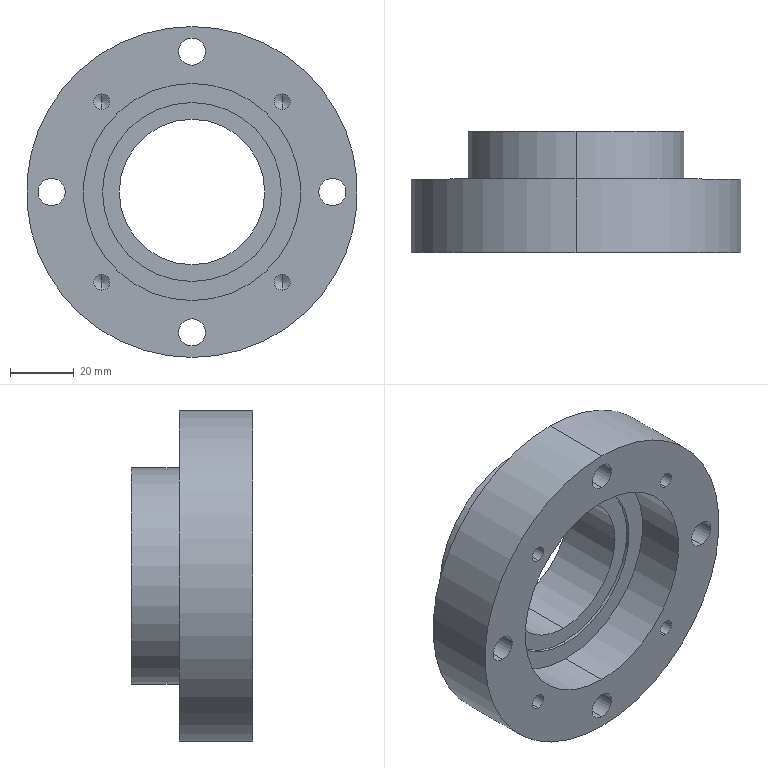Part | SolidWorks | features BaseBody 1 | 1 solid | 39 faces | box 103.7 x 38 x 103.7 mm | volume 146788 mm3 | cylinder 26 | cone 8 | plane 5 | commonest cylinder face diameters 5 x8 8.5 x8 45.6 x2 56.041 x2 67.7 x2 68 x2
STEP:
#1=CARTESIAN_POINT('',(0.,-38.,51.85));
#2=VERTEX_POINT('',#1);
#3=CARTESIAN_POINT('',(0.,-38.,-51.85));
#4=VERTEX_POINT('',#3);
#5=CARTESIAN_POINT('',(0.,-38.,0.));
#6=DIRECTION('',(0.,1.,0.));
#7=DIRECTION('',(0.,0.,1.));
#8=AXIS2_PLACEMENT_3D('',#5,#6,#7);
#9=CIRCLE('',#8,51.85);
#10=EDGE_CURVE('',#2,#4,#9,.T.);
#11=ORIENTED_EDGE('',*,*,#10,.T.);
#12=CARTESIAN_POINT('',(0.,-15.,-51.85));
#13=VERTEX_POINT('',#12);
#14=CARTESIAN_POINT('',(0.,-38.,-51.85));
#15=DIRECTION('',(0.,1.,0.));
#16=VECTOR('',#15,1000.);
#17=LINE('',#14,#16);
#18=EDGE_CURVE('',#4,#13,#17,.T.);
#19=ORIENTED_EDGE('',*,*,#18,.T.);
#20=CARTESIAN_POINT('',(0.,-15.,51.85));
#21=VERTEX_POINT('',#20);
#22=CARTESIAN_POINT('',(0.,-15.,0.));
#23=DIRECTION('',(0.,-1.,0.));
#24=DIRECTION('',(0.,0.,1.));
#25=AXIS2_PLACEMENT_3D('',#22,#23,#24);
#26=CIRCLE('',#25,51.85);
#27=EDGE_CURVE('',#13,#21,#26,.T.);
#28=ORIENTED_EDGE('',*,*,#27,.T.);
#29=CARTESIAN_POINT('',(0.,-38.,51.85));
#30=DIRECTION('',(0.,1.,0.));
#31=VECTOR('',#30,1000.);
#32=LINE('',#29,#31);
#33=EDGE_CURVE('',#2,#21,#32,.T.);
#34=ORIENTED_EDGE('',*,*,#33,.F.);
#35=EDGE_LOOP('',(#11,#19,#28,#34));
#36=FACE_OUTER_BOUND('',#35,.T.);
#37=CARTESIAN_POINT('',(0.,-38.,0.));
#38=DIRECTION('',(0.,1.,0.));
#39=DIRECTION('',(0.,0.,1.));
#40=AXIS2_PLACEMENT_3D('',#37,#38,#39);
#41=CYLINDRICAL_SURFACE('',#40,51.85);
#42=ADVANCED_FACE('',(#36),#41,.T.);
#43=CARTESIAN_POINT('',(0.,-15.,33.85));
#44=VERTEX_POINT('',#43);
#45=CARTESIAN_POINT('',(0.,-15.,-33.85));
#46=VERTEX_POINT('',#45);
#47=CARTESIAN_POINT('',(0.,-15.,0.));
#48=DIRECTION('',(0.,1.,0.));
#49=DIRECTION('',(0.,0.,1.));
#50=AXIS2_PLACEMENT_3D('',#47,#48,#49);
#51=CIRCLE('',#50,33.85);
#52=EDGE_CURVE('',#44,#46,#51,.T.);
#53=ORIENTED_EDGE('',*,*,#52,.T.);
#54=CARTESIAN_POINT('',(0.,0.,-33.85));
#55=VERTEX_POINT('',#54);
#56=CARTESIAN_POINT('',(0.,-15.,-33.85));
#57=DIRECTION('',(0.,1.,0.));
#58=VECTOR('',#57,1000.);
#59=LINE('',#56,#58);
#60=EDGE_CURVE('',#46,#55,#59,.T.);
#61=ORIENTED_EDGE('',*,*,#60,.T.);
#62=CARTESIAN_POINT('',(0.,0.,33.85));
#63=VERTEX_POINT('',#62);
#64=CARTESIAN_POINT('',(0.,0.,0.));
#65=DIRECTION('',(0.,-1.,0.));
#66=DIRECTION('',(0.,0.,1.));
#67=AXIS2_PLACEMENT_3D('',#64,#65,#66);
#68=CIRCLE('',#67,33.85);
#69=EDGE_CURVE('',#55,#63,#68,.T.);
#70=ORIENTED_EDGE('',*,*,#69,.T.);
#71=CARTESIAN_POINT('',(0.,-15.,33.85));
#72=DIRECTION('',(0.,1.,0.));
#73=VECTOR('',#72,1000.);
#74=LINE('',#71,#73);
#75=EDGE_CURVE('',#44,#63,#74,.T.);
#76=ORIENTED_EDGE('',*,*,#75,.F.);
#77=EDGE_LOOP('',(#53,#61,#70,#76));
#78=FACE_OUTER_BOUND('',#77,.T.);
#79=CARTESIAN_POINT('',(0.,-15.,0.));
#80=DIRECTION('',(0.,1.,0.));
#81=DIRECTION('',(0.,0.,1.));
#82=AXIS2_PLACEMENT_3D('',#79,#80,#81);
#83=CYLINDRICAL_SURFACE('',#82,33.85);
#84=ADVANCED_FACE('',(#78),#83,.T.);
#85=CARTESIAN_POINT('',(0.,-15.,39.75));
#86=VERTEX_POINT('',#85);
#87=CARTESIAN_POINT('',(0.,-15.,48.25));
#88=VERTEX_POINT('',#87);
#89=CARTESIAN_POINT('',(0.,-15.,44.));
#90=DIRECTION('',(0.,1.,0.));
#91=DIRECTION('',(0.,0.,-1.));
#92=AXIS2_PLACEMENT_3D('',#89,#90,#91);
#93=CIRCLE('',#92,4.25);
#94=EDGE_CURVE('',#86,#88,#93,.T.);
#95=ORIENTED_EDGE('',*,*,#94,.T.);
#96=CARTESIAN_POINT('',(0.,-38.,48.25));
#97=VERTEX_POINT('',#96);
#98=CARTESIAN_POINT('',(0.,-38.,48.25));
#99=DIRECTION('',(0.,-1.,0.));
#100=VECTOR('',#99,1000.);
#101=LINE('',#98,#100);
#102=EDGE_CURVE('',#88,#97,#101,.T.);
#103=ORIENTED_EDGE('',*,*,#102,.T.);
#104=CARTESIAN_POINT('',(0.,-38.,39.75));
#105=VERTEX_POINT('',#104);
#106=CARTESIAN_POINT('',(0.,-38.,44.));
#107=DIRECTION('',(0.,1.,0.));
#108=DIRECTION('',(0.,0.,-1.));
#109=AXIS2_PLACEMENT_3D('',#106,#107,#108);
#110=CIRCLE('',#109,4.25);
#111=EDGE_CURVE('',#105,#97,#110,.T.);
#112=ORIENTED_EDGE('',*,*,#111,.F.);
#113=CARTESIAN_POINT('',(0.,-38.,39.75));
#114=DIRECTION('',(0.,-1.,0.));
#115=VECTOR('',#114,1000.);
#116=LINE('',#113,#115);
#117=EDGE_CURVE('',#86,#105,#116,.T.);
#118=ORIENTED_EDGE('',*,*,#117,.F.);
#119=EDGE_LOOP('',(#95,#103,#112,#118));
#120=FACE_OUTER_BOUND('',#119,.T.);
#121=CARTESIAN_POINT('',(0.,-38.,44.));
#122=DIRECTION('',(0.,-1.,0.));
#123=DIRECTION('',(0.,0.,-1.));
#124=AXIS2_PLACEMENT_3D('',#121,#122,#123);
#125=CYLINDRICAL_SURFACE('',#124,4.25);
#126=ADVANCED_FACE('',(#120),#125,.F.);
#127=CARTESIAN_POINT('',(44.,-15.,-4.25));
#128=VERTEX_POINT('',#127);
#129=CARTESIAN_POINT('',(44.,-15.,4.25));
#130=VERTEX_POINT('',#129);
#131=CARTESIAN_POINT('',(44.,-15.,0.));
#132=DIRECTION('',(0.,1.,0.));
#133=DIRECTION('',(0.,0.,-1.));
#134=AXIS2_PLACEMENT_3D('',#131,#132,#133);
#135=CIRCLE('',#134,4.25);
#136=EDGE_CURVE('',#128,#130,#135,.T.);
#137=ORIENTED_EDGE('',*,*,#136,.T.);
#138=CARTESIAN_POINT('',(44.,-38.,4.25));
#139=VERTEX_POINT('',#138);
#140=CARTESIAN_POINT('',(44.,-38.,4.25));
#141=DIRECTION('',(0.,-1.,0.));
#142=VECTOR('',#141,1000.);
#143=LINE('',#140,#142);
#144=EDGE_CURVE('',#130,#139,#143,.T.);
#145=ORIENTED_EDGE('',*,*,#144,.T.);
#146=CARTESIAN_POINT('',(44.,-38.,-4.25));
#147=VERTEX_POINT('',#146);
#148=CARTESIAN_POINT('',(44.,-38.,0.));
#149=DIRECTION('',(0.,1.,0.));
#150=DIRECTION('',(0.,0.,-1.));
#151=AXIS2_PLACEMENT_3D('',#148,#149,#150);
#152=CIRCLE('',#151,4.25);
#153=EDGE_CURVE('',#147,#139,#152,.T.);
#154=ORIENTED_EDGE('',*,*,#153,.F.);
#155=CARTESIAN_POINT('',(44.,-38.,-4.25));
#156=DIRECTION('',(0.,-1.,0.));
#157=VECTOR('',#156,1000.);
#158=LINE('',#155,#157);
#159=EDGE_CURVE('',#128,#147,#158,.T.);
#160=ORIENTED_EDGE('',*,*,#159,.F.);
#161=EDGE_LOOP('',(#137,#145,#154,#160));
#162=FACE_OUTER_BOUND('',#161,.T.);
#163=CARTESIAN_POINT('',(44.,-38.,0.));
#164=DIRECTION('',(0.,-1.,0.));
#165=DIRECTION('',(0.,0.,-1.));
#166=AXIS2_PLACEMENT_3D('',#163,#164,#165);
#167=CYLINDRICAL_SURFACE('',#166,4.25);
#168=ADVANCED_FACE('',(#162),#167,.F.);
#169=CARTESIAN_POINT('',(0.,-15.,-48.25));
#170=VERTEX_POINT('',#169);
#171=CARTESIAN_POINT('',(0.,-15.,-39.75));
#172=VERTEX_POINT('',#171);
#173=CARTESIAN_POINT('',(0.,-15.,-44.));
#174=DIRECTION('',(0.,1.,0.));
#175=DIRECTION('',(0.,0.,-1.));
#176=AXIS2_PLACEMENT_3D('',#173,#174,#175);
#177=CIRCLE('',#176,4.25);
#178=EDGE_CURVE('',#170,#172,#177,.T.);
#179=ORIENTED_EDGE('',*,*,#178,.T.);
#180=CARTESIAN_POINT('',(0.,-38.,-39.75));
#181=VERTEX_POINT('',#180);
#182=CARTESIAN_POINT('',(0.,-38.,-39.75));
#183=DIRECTION('',(0.,-1.,0.));
#184=VECTOR('',#183,1000.);
#185=LINE('',#182,#184);
#186=EDGE_CURVE('',#172,#181,#185,.T.);
#187=ORIENTED_EDGE('',*,*,#186,.T.);
#188=CARTESIAN_POINT('',(0.,-38.,-48.25));
#189=VERTEX_POINT('',#188);
#190=CARTESIAN_POINT('',(0.,-38.,-44.));
#191=DIRECTION('',(0.,1.,0.));
#192=DIRECTION('',(0.,0.,-1.));
#193=AXIS2_PLACEMENT_3D('',#190,#191,#192);
#194=CIRCLE('',#193,4.25);
#195=EDGE_CURVE('',#189,#181,#194,.T.);
#196=ORIENTED_EDGE('',*,*,#195,.F.);
#197=CARTESIAN_POINT('',(0.,-38.,-48.25));
#198=DIRECTION('',(0.,-1.,0.));
#199=VECTOR('',#198,1000.);
#200=LINE('',#197,#199);
#201=EDGE_CURVE('',#170,#189,#200,.T.);
#202=ORIENTED_EDGE('',*,*,#201,.F.);
#203=EDGE_LOOP('',(#179,#187,#196,#202));
#204=FACE_OUTER_BOUND('',#203,.T.);
#205=CARTESIAN_POINT('',(0.,-38.,-44.));
#206=DIRECTION('',(0.,-1.,0.));
#207=DIRECTION('',(0.,0.,-1.));
#208=AXIS2_PLACEMENT_3D('',#205,#206,#207);
#209=CYLINDRICAL_SURFACE('',#208,4.25);
#210=ADVANCED_FACE('',(#204),#209,.F.);
#211=CARTESIAN_POINT('',(-44.,-15.,-4.25));
#212=VERTEX_POINT('',#211);
#213=CARTESIAN_POINT('',(-44.,-15.,4.25));
#214=VERTEX_POINT('',#213);
#215=CARTESIAN_POINT('',(-44.,-15.,0.));
#216=DIRECTION('',(0.,1.,0.));
#217=DIRECTION('',(0.,0.,-1.));
#218=AXIS2_PLACEMENT_3D('',#215,#216,#217);
#219=CIRCLE('',#218,4.25);
#220=EDGE_CURVE('',#212,#214,#219,.T.);
#221=ORIENTED_EDGE('',*,*,#220,.T.);
#222=CARTESIAN_POINT('',(-44.,-38.,4.25));
#223=VERTEX_POINT('',#222);
#224=CARTESIAN_POINT('',(-44.,-38.,4.25));
#225=DIRECTION('',(0.,-1.,0.));
#226=VECTOR('',#225,1000.);
#227=LINE('',#224,#226);
#228=EDGE_CURVE('',#214,#223,#227,.T.);
#229=ORIENTED_EDGE('',*,*,#228,.T.);
#230=CARTESIAN_POINT('',(-44.,-38.,-4.25));
#231=VERTEX_POINT('',#230);
#232=CARTESIAN_POINT('',(-44.,-38.,0.));
#233=DIRECTION('',(0.,1.,0.));
#234=DIRECTION('',(0.,0.,-1.));
#235=AXIS2_PLACEMENT_3D('',#232,#233,#234);
#236=CIRCLE('',#235,4.25);
#237=EDGE_CURVE('',#231,#223,#236,.T.);
#238=ORIENTED_EDGE('',*,*,#237,.F.);
#239=CARTESIAN_POINT('',(-44.,-38.,-4.25));
#240=DIRECTION('',(0.,-1.,0.));
#241=VECTOR('',#240,1000.);
#242=LINE('',#239,#241);
#243=EDGE_CURVE('',#212,#231,#242,.T.);
#244=ORIENTED_EDGE('',*,*,#243,.F.);
#245=EDGE_LOOP('',(#221,#229,#238,#244));
#246=FACE_OUTER_BOUND('',#245,.T.);
#247=CARTESIAN_POINT('',(-44.,-38.,0.));
#248=DIRECTION('',(0.,-1.,0.));
#249=DIRECTION('',(0.,0.,-1.));
#250=AXIS2_PLACEMENT_3D('',#247,#248,#249);
#251=CYLINDRICAL_SURFACE('',#250,4.25);
#252=ADVANCED_FACE('',(#246),#251,.F.);
#253=CARTESIAN_POINT('',(0.,-22.,34.));
#254=VERTEX_POINT('',#253);
#255=CARTESIAN_POINT('',(0.,-22.,-34.));
#256=VERTEX_POINT('',#255);
#257=CARTESIAN_POINT('',(0.,-22.,0.));
#258=DIRECTION('',(0.,-1.,0.));
#259=DIRECTION('',(0.,0.,-1.));
#260=AXIS2_PLACEMENT_3D('',#257,#258,#259);
#261=CIRCLE('',#260,34.);
#262=EDGE_CURVE('',#254,#256,#261,.T.);
#263=ORIENTED_EDGE('',*,*,#262,.F.);
#264=CARTESIAN_POINT('',(0.,-38.,34.));
#265=VERTEX_POINT('',#264);
#266=CARTESIAN_POINT('',(0.,-22.,34.));
#267=DIRECTION('',(0.,-1.,0.));
#268=VECTOR('',#267,1000.);
#269=LINE('',#266,#268);
#270=EDGE_CURVE('',#254,#265,#269,.T.);
#271=ORIENTED_EDGE('',*,*,#270,.T.);
#272=CARTESIAN_POINT('',(0.,-38.,-34.));
#273=VERTEX_POINT('',#272);
#274=CARTESIAN_POINT('',(0.,-38.,0.));
#275=DIRECTION('',(0.,1.,0.));
#276=DIRECTION('',(0.,0.,-1.));
#277=AXIS2_PLACEMENT_3D('',#274,#275,#276);
#278=CIRCLE('',#277,34.);
#279=EDGE_CURVE('',#273,#265,#278,.T.);
#280=ORIENTED_EDGE('',*,*,#279,.F.);
#281=CARTESIAN_POINT('',(0.,-22.,-34.));
#282=DIRECTION('',(0.,-1.,0.));
#283=VECTOR('',#282,1000.);
#284=LINE('',#281,#283);
#285=EDGE_CURVE('',#256,#273,#284,.T.);
#286=ORIENTED_EDGE('',*,*,#285,.F.);
#287=EDGE_LOOP('',(#263,#271,#280,#286));
#288=FACE_OUTER_BOUND('',#287,.T.);
#289=CARTESIAN_POINT('',(0.,-22.,0.));
#290=DIRECTION('',(0.,-1.,0.));
#291=DIRECTION('',(0.,0.,-1.));
#292=AXIS2_PLACEMENT_3D('',#289,#290,#291);
#293=CYLINDRICAL_SURFACE('',#292,34.);
#294=ADVANCED_FACE('',(#288),#293,.F.);
#295=CARTESIAN_POINT('',(-28.284,-21.,30.784));
#296=VERTEX_POINT('',#295);
#297=CARTESIAN_POINT('',(-28.284,-21.,25.784));
#298=VERTEX_POINT('',#297);
#299=CARTESIAN_POINT('',(-28.284,-21.,28.284));
#300=DIRECTION('',(0.,-1.,0.));
#301=DIRECTION('',(0.,0.,-1.));
#302=AXIS2_PLACEMENT_3D('',#299,#300,#301);
#303=CIRCLE('',#302,2.5);
#304=EDGE_CURVE('',#296,#298,#303,.T.);
#305=ORIENTED_EDGE('',*,*,#304,.F.);
#306=CARTESIAN_POINT('',(-28.284,-38.,30.784));
#307=VERTEX_POINT('',#306);
#308=CARTESIAN_POINT('',(-28.284,-38.,30.784));
#309=DIRECTION('',(0.,-1.,0.));
#310=VECTOR('',#309,1000.);
#311=LINE('',#308,#310);
#312=EDGE_CURVE('',#296,#307,#311,.T.);
#313=ORIENTED_EDGE('',*,*,#312,.T.);
#314=CARTESIAN_POINT('',(-28.284,-38.,25.784));
#315=VERTEX_POINT('',#314);
#316=CARTESIAN_POINT('',(-28.284,-38.,28.284));
#317=DIRECTION('',(0.,1.,0.));
#318=DIRECTION('',(0.,0.,-1.));
#319=AXIS2_PLACEMENT_3D('',#316,#317,#318);
#320=CIRCLE('',#319,2.5);
#321=EDGE_CURVE('',#315,#307,#320,.T.);
#322=ORIENTED_EDGE('',*,*,#321,.F.);
#323=CARTESIAN_POINT('',(-28.284,-38.,25.784));
#324=DIRECTION('',(0.,-1.,0.));
#325=VECTOR('',#324,1000.);
#326=LINE('',#323,#325);
#327=EDGE_CURVE('',#298,#315,#326,.T.);
#328=ORIENTED_EDGE('',*,*,#327,.F.);
#329=EDGE_LOOP('',(#305,#313,#322,#328));
#330=FACE_OUTER_BOUND('',#329,.T.);
#331=CARTESIAN_POINT('',(-28.284,-38.,28.284));
#332=DIRECTION('',(0.,-1.,0.));
#333=DIRECTION('',(0.,0.,-1.));
#334=AXIS2_PLACEMENT_3D('',#331,#332,#333);
#335=CYLINDRICAL_SURFACE('',#334,2.5);
#336=ADVANCED_FACE('',(#330),#335,.F.);
#337=CARTESIAN_POINT('',(28.284,-21.,30.784));
#338=VERTEX_POINT('',#337);
#339=CARTESIAN_POINT('',(28.284,-21.,25.784));
#340=VERTEX_POINT('',#339);
#341=CARTESIAN_POINT('',(28.284,-21.,28.284));
#342=DIRECTION('',(0.,-1.,0.));
#343=DIRECTION('',(0.,0.,-1.));
#344=AXIS2_PLACEMENT_3D('',#341,#342,#343);
#345=CIRCLE('',#344,2.5);
#346=EDGE_CURVE('',#338,#340,#345,.T.);
#347=ORIENTED_EDGE('',*,*,#346,.F.);
#348=CARTESIAN_POINT('',(28.284,-38.,30.784));
#349=VERTEX_POINT('',#348);
#350=CARTESIAN_POINT('',(28.284,-38.,30.784));
#351=DIRECTION('',(0.,-1.,0.));
#352=VECTOR('',#351,1000.);
#353=LINE('',#350,#352);
#354=EDGE_CURVE('',#338,#349,#353,.T.);
#355=ORIENTED_EDGE('',*,*,#354,.T.);
#356=CARTESIAN_POINT('',(28.284,-38.,25.784));
#357=VERTEX_POINT('',#356);
#358=CARTESIAN_POINT('',(28.284,-38.,28.284));
#359=DIRECTION('',(0.,1.,0.));
#360=DIRECTION('',(0.,0.,-1.));
#361=AXIS2_PLACEMENT_3D('',#358,#359,#360);
#362=CIRCLE('',#361,2.5);
#363=EDGE_CURVE('',#357,#349,#362,.T.);
#364=ORIENTED_EDGE('',*,*,#363,.F.);
#365=CARTESIAN_POINT('',(28.284,-38.,25.784));
#366=DIRECTION('',(0.,-1.,0.));
#367=VECTOR('',#366,1000.);
#368=LINE('',#365,#367);
#369=EDGE_CURVE('',#340,#357,#368,.T.);
#370=ORIENTED_EDGE('',*,*,#369,.F.);
#371=EDGE_LOOP('',(#347,#355,#364,#370));
#372=FACE_OUTER_BOUND('',#371,.T.);
#373=CARTESIAN_POINT('',(28.284,-38.,28.284));
#374=DIRECTION('',(0.,-1.,0.));
#375=DIRECTION('',(0.,0.,-1.));
#376=AXIS2_PLACEMENT_3D('',#373,#374,#375);
#377=CYLINDRICAL_SURFACE('',#376,2.5);
#378=ADVANCED_FACE('',(#372),#377,.F.);
#379=CARTESIAN_POINT('',(28.284,-21.,-25.784));
#380=VERTEX_POINT('',#379);
#381=CARTESIAN_POINT('',(28.284,-21.,-30.784));
#382=VERTEX_POINT('',#381);
#383=CARTESIAN_POINT('',(28.284,-21.,-28.284));
#384=DIRECTION('',(0.,-1.,0.));
#385=DIRECTION('',(0.,0.,-1.));
#386=AXIS2_PLACEMENT_3D('',#383,#384,#385);
#387=CIRCLE('',#386,2.5);
#388=EDGE_CURVE('',#380,#382,#387,.T.);
#389=ORIENTED_EDGE('',*,*,#388,.F.);
#390=CARTESIAN_POINT('',(28.284,-38.,-25.784));
#391=VERTEX_POINT('',#390);
#392=CARTESIAN_POINT('',(28.284,-38.,-25.784));
#393=DIRECTION('',(0.,-1.,0.));
#394=VECTOR('',#393,1000.);
#395=LINE('',#392,#394);
#396=EDGE_CURVE('',#380,#391,#395,.T.);
#397=ORIENTED_EDGE('',*,*,#396,.T.);
#398=CARTESIAN_POINT('',(28.284,-38.,-30.784));
#399=VERTEX_POINT('',#398);
#400=CARTESIAN_POINT('',(28.284,-38.,-28.284));
#401=DIRECTION('',(0.,1.,0.));
#402=DIRECTION('',(0.,0.,-1.));
#403=AXIS2_PLACEMENT_3D('',#400,#401,#402);
#404=CIRCLE('',#403,2.5);
#405=EDGE_CURVE('',#399,#391,#404,.T.);
#406=ORIENTED_EDGE('',*,*,#405,.F.);
#407=CARTESIAN_POINT('',(28.284,-38.,-30.784));
#408=DIRECTION('',(0.,-1.,0.));
#409=VECTOR('',#408,1000.);
#410=LINE('',#407,#409);
#411=EDGE_CURVE('',#382,#399,#410,.T.);
#412=ORIENTED_EDGE('',*,*,#411,.F.);
#413=EDGE_LOOP('',(#389,#397,#406,#412));
#414=FACE_OUTER_BOUND('',#413,.T.);
#415=CARTESIAN_POINT('',(28.284,-38.,-28.284));
#416=DIRECTION('',(0.,-1.,0.));
#417=DIRECTION('',(0.,0.,-1.));
#418=AXIS2_PLACEMENT_3D('',#415,#416,#417);
#419=CYLINDRICAL_SURFACE('',#418,2.5);
#420=ADVANCED_FACE('',(#414),#419,.F.);
#421=CARTESIAN_POINT('',(-28.284,-21.,-25.784));
#422=VERTEX_POINT('',#421);
#423=CARTESIAN_POINT('',(-28.284,-21.,-30.784));
#424=VERTEX_POINT('',#423);
#425=CARTESIAN_POINT('',(-28.284,-21.,-28.284));
#426=DIRECTION('',(0.,-1.,0.));
#427=DIRECTION('',(0.,0.,-1.));
#428=AXIS2_PLACEMENT_3D('',#425,#426,#427);
#429=CIRCLE('',#428,2.5);
#430=EDGE_CURVE('',#422,#424,#429,.T.);
#431=ORIENTED_EDGE('',*,*,#430,.F.);
#432=CARTESIAN_POINT('',(-28.284,-38.,-25.784));
#433=VERTEX_POINT('',#432);
#434=CARTESIAN_POINT('',(-28.284,-38.,-25.784));
#435=DIRECTION('',(0.,-1.,0.));
#436=VECTOR('',#435,1000.);
#437=LINE('',#434,#436);
#438=EDGE_CURVE('',#422,#433,#437,.T.);
#439=ORIENTED_EDGE('',*,*,#438,.T.);
#440=CARTESIAN_POINT('',(-28.284,-38.,-30.784));
#441=VERTEX_POINT('',#440);
#442=CARTESIAN_POINT('',(-28.284,-38.,-28.284));
#443=DIRECTION('',(0.,1.,0.));
#444=DIRECTION('',(0.,0.,-1.));
#445=AXIS2_PLACEMENT_3D('',#442,#443,#444);
#446=CIRCLE('',#445,2.5);
#447=EDGE_CURVE('',#441,#433,#446,.T.);
#448=ORIENTED_EDGE('',*,*,#447,.F.);
#449=CARTESIAN_POINT('',(-28.284,-38.,-30.784));
#450=DIRECTION('',(0.,-1.,0.));
#451=VECTOR('',#450,1000.);
#452=LINE('',#449,#451);
#453=EDGE_CURVE('',#424,#441,#452,.T.);
#454=ORIENTED_EDGE('',*,*,#453,.F.);
#455=EDGE_LOOP('',(#431,#439,#448,#454));
#456=FACE_OUTER_BOUND('',#455,.T.);
#457=CARTESIAN_POINT('',(-28.284,-38.,-28.284));
#458=DIRECTION('',(0.,-1.,0.));
#459=DIRECTION('',(0.,0.,-1.));
#460=AXIS2_PLACEMENT_3D('',#457,#458,#459);
#461=CYLINDRICAL_SURFACE('',#460,2.5);
#462=ADVANCED_FACE('',(#456),#461,.F.);
#463=CARTESIAN_POINT('',(0.,-21.,-22.8));
#464=VERTEX_POINT('',#463);
#465=CARTESIAN_POINT('',(0.,-21.,22.8));
#466=VERTEX_POINT('',#465);
#467=CARTESIAN_POINT('',(0.,-21.,0.));
#468=DIRECTION('',(0.,1.,0.));
#469=DIRECTION('',(0.,0.,1.));
#470=AXIS2_PLACEMENT_3D('',#467,#468,#469);
#471=CIRCLE('',#470,22.8);
#472=EDGE_CURVE('',#464,#466,#471,.T.);
#473=ORIENTED_EDGE('',*,*,#472,.F.);
#474=CARTESIAN_POINT('',(0.,0.,-22.8));
#475=VERTEX_POINT('',#474);
#476=CARTESIAN_POINT('',(0.,-15.,-22.8));
#477=DIRECTION('',(0.,1.,0.));
#478=VECTOR('',#477,1000.);
#479=LINE('',#476,#478);
#480=EDGE_CURVE('',#464,#475,#479,.T.);
#481=ORIENTED_EDGE('',*,*,#480,.T.);
#482=CARTESIAN_POINT('',(0.,0.,22.8));
#483=VERTEX_POINT('',#482);
#484=CARTESIAN_POINT('',(0.,0.,0.));
#485=DIRECTION('',(0.,-1.,0.));
#486=DIRECTION('',(0.,0.,1.));
#487=AXIS2_PLACEMENT_3D('',#484,#485,#486);
#488=CIRCLE('',#487,22.8);
#489=EDGE_CURVE('',#483,#475,#488,.T.);
#490=ORIENTED_EDGE('',*,*,#489,.F.);
#491=CARTESIAN_POINT('',(0.,-15.,22.8));
#492=DIRECTION('',(0.,1.,0.));
#493=VECTOR('',#492,1000.);
#494=LINE('',#491,#493);
#495=EDGE_CURVE('',#466,#483,#494,.T.);
#496=ORIENTED_EDGE('',*,*,#495,.F.);
#497=EDGE_LOOP('',(#473,#481,#490,#496));
#498=FACE_OUTER_BOUND('',#497,.T.);
#499=CARTESIAN_POINT('',(0.,-15.,0.));
#500=DIRECTION('',(0.,1.,0.));
#501=DIRECTION('',(0.,0.,1.));
#502=AXIS2_PLACEMENT_3D('',#499,#500,#501);
#503=CYLINDRICAL_SURFACE('',#502,22.8);
#504=ADVANCED_FACE('',(#498),#503,.F.);
#505=CARTESIAN_POINT('',(-28.284,-19.498,28.284));
#506=VERTEX_POINT('',#505);
#507=CARTESIAN_POINT('',(-28.284,-21.,25.784));
#508=DIRECTION('',(0.,-0.515,-0.8572));
#509=VECTOR('',#508,1000.);
#510=LINE('',#507,#509);
#511=EDGE_CURVE('',#506,#298,#510,.T.);
#512=ORIENTED_EDGE('',*,*,#511,.F.);
#513=CARTESIAN_POINT('',(-28.284,-21.,30.784));
#514=DIRECTION('',(0.,-0.515,0.8572));
#515=VECTOR('',#514,1000.);
#516=LINE('',#513,#515);
#517=EDGE_CURVE('',#506,#296,#516,.T.);
#518=ORIENTED_EDGE('',*,*,#517,.T.);
#519=ORIENTED_EDGE('',*,*,#304,.T.);
#520=EDGE_LOOP('',(#512,#518,#519));
#521=FACE_OUTER_BOUND('',#520,.T.);
#522=CARTESIAN_POINT('',(-28.284,-21.,28.284));
#523=DIRECTION('',(0.,-1.,0.));
#524=DIRECTION('',(0.,0.,-1.));
#525=AXIS2_PLACEMENT_3D('',#522,#523,#524);
#526=CONICAL_SURFACE('',#525,2.5,1.03);
#527=ADVANCED_FACE('',(#521),#526,.F.);
#528=CARTESIAN_POINT('',(28.284,-19.498,28.284));
#529=VERTEX_POINT('',#528);
#530=CARTESIAN_POINT('',(28.284,-21.,25.784));
#531=DIRECTION('',(0.,-0.515,-0.8572));
#532=VECTOR('',#531,1000.);
#533=LINE('',#530,#532);
#534=EDGE_CURVE('',#529,#340,#533,.T.);
#535=ORIENTED_EDGE('',*,*,#534,.F.);
#536=CARTESIAN_POINT('',(28.284,-21.,30.784));
#537=DIRECTION('',(0.,-0.515,0.8572));
#538=VECTOR('',#537,1000.);
#539=LINE('',#536,#538);
#540=EDGE_CURVE('',#529,#338,#539,.T.);
#541=ORIENTED_EDGE('',*,*,#540,.T.);
#542=ORIENTED_EDGE('',*,*,#346,.T.);
#543=EDGE_LOOP('',(#535,#541,#542));
#544=FACE_OUTER_BOUND('',#543,.T.);
#545=CARTESIAN_POINT('',(28.284,-21.,28.284));
#546=DIRECTION('',(0.,-1.,0.));
#547=DIRECTION('',(0.,0.,-1.));
#548=AXIS2_PLACEMENT_3D('',#545,#546,#547);
#549=CONICAL_SURFACE('',#548,2.5,1.03);
#550=ADVANCED_FACE('',(#544),#549,.F.);
#551=CARTESIAN_POINT('',(28.284,-19.498,-28.284));
#552=VERTEX_POINT('',#551);
#553=CARTESIAN_POINT('',(28.284,-21.,-30.784));
#554=DIRECTION('',(0.,-0.515,-0.8572));
#555=VECTOR('',#554,1000.);
#556=LINE('',#553,#555);
#557=EDGE_CURVE('',#552,#382,#556,.T.);
#558=ORIENTED_EDGE('',*,*,#557,.F.);
#559=CARTESIAN_POINT('',(28.284,-21.,-25.784));
#560=DIRECTION('',(0.,-0.515,0.8572));
#561=VECTOR('',#560,1000.);
#562=LINE('',#559,#561);
#563=EDGE_CURVE('',#552,#380,#562,.T.);
#564=ORIENTED_EDGE('',*,*,#563,.T.);
#565=ORIENTED_EDGE('',*,*,#388,.T.);
#566=EDGE_LOOP('',(#558,#564,#565));
#567=FACE_OUTER_BOUND('',#566,.T.);
#568=CARTESIAN_POINT('',(28.284,-21.,-28.284));
#569=DIRECTION('',(0.,-1.,0.));
#570=DIRECTION('',(0.,0.,-1.));
#571=AXIS2_PLACEMENT_3D('',#568,#569,#570);
#572=CONICAL_SURFACE('',#571,2.5,1.03);
#573=ADVANCED_FACE('',(#567),#572,.F.);
#574=CARTESIAN_POINT('',(-28.284,-19.498,-28.284));
#575=VERTEX_POINT('',#574);
#576=CARTESIAN_POINT('',(-28.284,-21.,-30.784));
#577=DIRECTION('',(0.,-0.515,-0.8572));
#578=VECTOR('',#577,1000.);
#579=LINE('',#576,#578);
#580=EDGE_CURVE('',#575,#424,#579,.T.);
#581=ORIENTED_EDGE('',*,*,#580,.F.);
#582=CARTESIAN_POINT('',(-28.284,-21.,-25.784));
#583=DIRECTION('',(0.,-0.515,0.8572));
#584=VECTOR('',#583,1000.);
#585=LINE('',#582,#584);
#586=EDGE_CURVE('',#575,#422,#585,.T.);
#587=ORIENTED_EDGE('',*,*,#586,.T.);
#588=ORIENTED_EDGE('',*,*,#430,.T.);
#589=EDGE_LOOP('',(#581,#587,#588));
#590=FACE_OUTER_BOUND('',#589,.T.);
#591=CARTESIAN_POINT('',(-28.284,-21.,-28.284));
#592=DIRECTION('',(0.,-1.,0.));
#593=DIRECTION('',(0.,0.,-1.));
#594=AXIS2_PLACEMENT_3D('',#591,#592,#593);
#595=CONICAL_SURFACE('',#594,2.5,1.03);
#596=ADVANCED_FACE('',(#590),#595,.F.);
#597=CARTESIAN_POINT('',(0.,-21.,28.02));
#598=VERTEX_POINT('',#597);
#599=CARTESIAN_POINT('',(0.,-21.,-28.02));
#600=VERTEX_POINT('',#599);
#601=CARTESIAN_POINT('',(0.,-21.,0.));
#602=DIRECTION('',(0.,-1.,0.));
#603=DIRECTION('',(0.,0.,-1.));
#604=AXIS2_PLACEMENT_3D('',#601,#602,#603);
#605=CIRCLE('',#604,28.02);
#606=EDGE_CURVE('',#598,#600,#605,.T.);
#607=ORIENTED_EDGE('',*,*,#606,.F.);
#608=CARTESIAN_POINT('',(0.,-22.,28.02));
#609=VERTEX_POINT('',#608);
#610=CARTESIAN_POINT('',(0.,-21.,28.02));
#611=DIRECTION('',(0.,-1.,0.));
#612=VECTOR('',#611,1000.);
#613=LINE('',#610,#612);
#614=EDGE_CURVE('',#598,#609,#613,.T.);
#615=ORIENTED_EDGE('',*,*,#614,.T.);
#616=CARTESIAN_POINT('',(0.,-22.,-28.02));
#617=VERTEX_POINT('',#616);
#618=CARTESIAN_POINT('',(0.,-22.,0.));
#619=DIRECTION('',(0.,1.,0.));
#620=DIRECTION('',(0.,0.,-1.));
#621=AXIS2_PLACEMENT_3D('',#618,#619,#620);
#622=CIRCLE('',#621,28.02);
#623=EDGE_CURVE('',#617,#609,#622,.T.);
#624=ORIENTED_EDGE('',*,*,#623,.F.);
#625=CARTESIAN_POINT('',(0.,-21.,-28.02));
#626=DIRECTION('',(0.,-1.,0.));
#627=VECTOR('',#626,1000.);
#628=LINE('',#625,#627);
#629=EDGE_CURVE('',#600,#617,#628,.T.);
#630=ORIENTED_EDGE('',*,*,#629,.F.);
#631=EDGE_LOOP('',(#607,#615,#624,#630));
#632=FACE_OUTER_BOUND('',#631,.T.);
#633=CARTESIAN_POINT('',(0.,-21.,0.));
#634=DIRECTION('',(0.,-1.,0.));
#635=DIRECTION('',(0.,0.,-1.));
#636=AXIS2_PLACEMENT_3D('',#633,#634,#635);
#637=CYLINDRICAL_SURFACE('',#636,28.02);
#638=ADVANCED_FACE('',(#632),#637,.F.);
#639=CARTESIAN_POINT('',(0.,-15.,0.));
#640=DIRECTION('',(0.,-1.,0.));
#641=DIRECTION('',(0.,0.,1.));
#642=AXIS2_PLACEMENT_3D('',#639,#640,#641);
#643=CIRCLE('',#642,51.85);
#644=EDGE_CURVE('',#21,#13,#643,.T.);
#645=ORIENTED_EDGE('',*,*,#644,.F.);
#646=ORIENTED_EDGE('',*,*,#27,.F.);
#647=EDGE_LOOP('',(#645,#646));
#648=FACE_OUTER_BOUND('',#647,.T.);
#649=ORIENTED_EDGE('',*,*,#52,.F.);
#650=CARTESIAN_POINT('',(0.,-15.,0.));
#651=DIRECTION('',(0.,1.,0.));
#652=DIRECTION('',(0.,0.,1.));
#653=AXIS2_PLACEMENT_3D('',#650,#651,#652);
#654=CIRCLE('',#653,33.85);
#655=EDGE_CURVE('',#46,#44,#654,.T.);
#656=ORIENTED_EDGE('',*,*,#655,.F.);
#657=EDGE_LOOP('',(#649,#656));
#658=FACE_BOUND('',#657,.T.);
#659=ORIENTED_EDGE('',*,*,#94,.F.);
#660=CARTESIAN_POINT('',(0.,-15.,44.));
#661=DIRECTION('',(0.,1.,0.));
#662=DIRECTION('',(0.,0.,-1.));
#663=AXIS2_PLACEMENT_3D('',#660,#661,#662);
#664=CIRCLE('',#663,4.25);
#665=EDGE_CURVE('',#88,#86,#664,.T.);
#666=ORIENTED_EDGE('',*,*,#665,.F.);
#667=EDGE_LOOP('',(#659,#666));
#668=FACE_BOUND('',#667,.T.);
#669=ORIENTED_EDGE('',*,*,#136,.F.);
#670=CARTESIAN_POINT('',(44.,-15.,0.));
#671=DIRECTION('',(0.,1.,0.));
#672=DIRECTION('',(0.,0.,-1.));
#673=AXIS2_PLACEMENT_3D('',#670,#671,#672);
#674=CIRCLE('',#673,4.25);
#675=EDGE_CURVE('',#130,#128,#674,.T.);
#676=ORIENTED_EDGE('',*,*,#675,.F.);
#677=EDGE_LOOP('',(#669,#676));
#678=FACE_BOUND('',#677,.T.);
#679=ORIENTED_EDGE('',*,*,#178,.F.);
#680=CARTESIAN_POINT('',(0.,-15.,-44.));
#681=DIRECTION('',(0.,1.,0.));
#682=DIRECTION('',(0.,0.,-1.));
#683=AXIS2_PLACEMENT_3D('',#680,#681,#682);
#684=CIRCLE('',#683,4.25);
#685=EDGE_CURVE('',#172,#170,#684,.T.);
#686=ORIENTED_EDGE('',*,*,#685,.F.);
#687=EDGE_LOOP('',(#679,#686));
#688=FACE_BOUND('',#687,.T.);
#689=ORIENTED_EDGE('',*,*,#220,.F.);
#690=CARTESIAN_POINT('',(-44.,-15.,0.));
#691=DIRECTION('',(0.,1.,0.));
#692=DIRECTION('',(0.,0.,-1.));
#693=AXIS2_PLACEMENT_3D('',#690,#691,#692);
#694=CIRCLE('',#693,4.25);
#695=EDGE_CURVE('',#214,#212,#694,.T.);
#696=ORIENTED_EDGE('',*,*,#695,.F.);
#697=EDGE_LOOP('',(#689,#696));
#698=FACE_BOUND('',#697,.T.);
#699=CARTESIAN_POINT('',(0.,-15.,0.));
#700=DIRECTION('',(0.,-1.,0.));
#701=DIRECTION('',(0.,0.,-1.));
#702=AXIS2_PLACEMENT_3D('',#699,#700,#701);
#703=PLANE('',#702);
#704=ADVANCED_FACE('',(#648,#658,#668,#678,#688,#698),#703,.F.);
#705=ORIENTED_EDGE('',*,*,#18,.F.);
#706=CARTESIAN_POINT('',(0.,-38.,0.));
#707=DIRECTION('',(0.,1.,0.));
#708=DIRECTION('',(0.,0.,1.));
#709=AXIS2_PLACEMENT_3D('',#706,#707,#708);
#710=CIRCLE('',#709,51.85);
#711=EDGE_CURVE('',#4,#2,#710,.T.);
#712=ORIENTED_EDGE('',*,*,#711,.T.);
#713=ORIENTED_EDGE('',*,*,#33,.T.);
#714=ORIENTED_EDGE('',*,*,#644,.T.);
#715=EDGE_LOOP('',(#705,#712,#713,#714));
#716=FACE_OUTER_BOUND('',#715,.T.);
#717=CARTESIAN_POINT('',(0.,-38.,0.));
#718=DIRECTION('',(0.,1.,0.));
#719=DIRECTION('',(0.,0.,1.));
#720=AXIS2_PLACEMENT_3D('',#717,#718,#719);
#721=CYLINDRICAL_SURFACE('',#720,51.85);
#722=ADVANCED_FACE('',(#716),#721,.T.);
#723=ORIENTED_EDGE('',*,*,#60,.F.);
#724=ORIENTED_EDGE('',*,*,#655,.T.);
#725=ORIENTED_EDGE('',*,*,#75,.T.);
#726=CARTESIAN_POINT('',(0.,0.,0.));
#727=DIRECTION('',(0.,-1.,0.));
#728=DIRECTION('',(0.,0.,1.));
#729=AXIS2_PLACEMENT_3D('',#726,#727,#728);
#730=CIRCLE('',#729,33.85);
#731=EDGE_CURVE('',#63,#55,#730,.T.);
#732=ORIENTED_EDGE('',*,*,#731,.T.);
#733=EDGE_LOOP('',(#723,#724,#725,#732));
#734=FACE_OUTER_BOUND('',#733,.T.);
#735=CARTESIAN_POINT('',(0.,-15.,0.));
#736=DIRECTION('',(0.,1.,0.));
#737=DIRECTION('',(0.,0.,1.));
#738=AXIS2_PLACEMENT_3D('',#735,#736,#737);
#739=CYLINDRICAL_SURFACE('',#738,33.85);
#740=ADVANCED_FACE('',(#734),#739,.T.);
#741=ORIENTED_EDGE('',*,*,#102,.F.);
#742=ORIENTED_EDGE('',*,*,#665,.T.);
#743=ORIENTED_EDGE('',*,*,#117,.T.);
#744=CARTESIAN_POINT('',(0.,-38.,44.));
#745=DIRECTION('',(0.,1.,0.));
#746=DIRECTION('',(0.,0.,-1.));
#747=AXIS2_PLACEMENT_3D('',#744,#745,#746);
#748=CIRCLE('',#747,4.25);
#749=EDGE_CURVE('',#97,#105,#748,.T.);
#750=ORIENTED_EDGE('',*,*,#749,.F.);
#751=EDGE_LOOP('',(#741,#742,#743,#750));
#752=FACE_OUTER_BOUND('',#751,.T.);
#753=CARTESIAN_POINT('',(0.,-38.,44.));
#754=DIRECTION('',(0.,-1.,0.));
#755=DIRECTION('',(0.,0.,-1.));
#756=AXIS2_PLACEMENT_3D('',#753,#754,#755);
#757=CYLINDRICAL_SURFACE('',#756,4.25);
#758=ADVANCED_FACE('',(#752),#757,.F.);
#759=ORIENTED_EDGE('',*,*,#144,.F.);
#760=ORIENTED_EDGE('',*,*,#675,.T.);
#761=ORIENTED_EDGE('',*,*,#159,.T.);
#762=CARTESIAN_POINT('',(44.,-38.,0.));
#763=DIRECTION('',(0.,1.,0.));
#764=DIRECTION('',(0.,0.,-1.));
#765=AXIS2_PLACEMENT_3D('',#762,#763,#764);
#766=CIRCLE('',#765,4.25);
#767=EDGE_CURVE('',#139,#147,#766,.T.);
#768=ORIENTED_EDGE('',*,*,#767,.F.);
#769=EDGE_LOOP('',(#759,#760,#761,#768));
#770=FACE_OUTER_BOUND('',#769,.T.);
#771=CARTESIAN_POINT('',(44.,-38.,0.));
#772=DIRECTION('',(0.,-1.,0.));
#773=DIRECTION('',(0.,0.,-1.));
#774=AXIS2_PLACEMENT_3D('',#771,#772,#773);
#775=CYLINDRICAL_SURFACE('',#774,4.25);
#776=ADVANCED_FACE('',(#770),#775,.F.);
#777=ORIENTED_EDGE('',*,*,#186,.F.);
#778=ORIENTED_EDGE('',*,*,#685,.T.);
#779=ORIENTED_EDGE('',*,*,#201,.T.);
#780=CARTESIAN_POINT('',(0.,-38.,-44.));
#781=DIRECTION('',(0.,1.,0.));
#782=DIRECTION('',(0.,0.,-1.));
#783=AXIS2_PLACEMENT_3D('',#780,#781,#782);
#784=CIRCLE('',#783,4.25);
#785=EDGE_CURVE('',#181,#189,#784,.T.);
#786=ORIENTED_EDGE('',*,*,#785,.F.);
#787=EDGE_LOOP('',(#777,#778,#779,#786));
#788=FACE_OUTER_BOUND('',#787,.T.);
#789=CARTESIAN_POINT('',(0.,-38.,-44.));
#790=DIRECTION('',(0.,-1.,0.));
#791=DIRECTION('',(0.,0.,-1.));
#792=AXIS2_PLACEMENT_3D('',#789,#790,#791);
#793=CYLINDRICAL_SURFACE('',#792,4.25);
#794=ADVANCED_FACE('',(#788),#793,.F.);
#795=ORIENTED_EDGE('',*,*,#228,.F.);
#796=ORIENTED_EDGE('',*,*,#695,.T.);
#797=ORIENTED_EDGE('',*,*,#243,.T.);
#798=CARTESIAN_POINT('',(-44.,-38.,0.));
#799=DIRECTION('',(0.,1.,0.));
#800=DIRECTION('',(0.,0.,-1.));
#801=AXIS2_PLACEMENT_3D('',#798,#799,#800);
#802=CIRCLE('',#801,4.25);
#803=EDGE_CURVE('',#223,#231,#802,.T.);
#804=ORIENTED_EDGE('',*,*,#803,.F.);
#805=EDGE_LOOP('',(#795,#796,#797,#804));
#806=FACE_OUTER_BOUND('',#805,.T.);
#807=CARTESIAN_POINT('',(-44.,-38.,0.));
#808=DIRECTION('',(0.,-1.,0.));
#809=DIRECTION('',(0.,0.,-1.));
#810=AXIS2_PLACEMENT_3D('',#807,#808,#809);
#811=CYLINDRICAL_SURFACE('',#810,4.25);
#812=ADVANCED_FACE('',(#806),#811,.F.);
#813=ORIENTED_EDGE('',*,*,#10,.F.);
#814=ORIENTED_EDGE('',*,*,#711,.F.);
#815=EDGE_LOOP('',(#813,#814));
#816=FACE_OUTER_BOUND('',#815,.T.);
#817=ORIENTED_EDGE('',*,*,#279,.T.);
#818=CARTESIAN_POINT('',(0.,-38.,0.));
#819=DIRECTION('',(0.,1.,0.));
#820=DIRECTION('',(0.,0.,-1.));
#821=AXIS2_PLACEMENT_3D('',#818,#819,#820);
#822=CIRCLE('',#821,34.);
#823=EDGE_CURVE('',#265,#273,#822,.T.);
#824=ORIENTED_EDGE('',*,*,#823,.T.);
#825=EDGE_LOOP('',(#817,#824));
#826=FACE_BOUND('',#825,.T.);
#827=ORIENTED_EDGE('',*,*,#111,.T.);
#828=ORIENTED_EDGE('',*,*,#749,.T.);
#829=EDGE_LOOP('',(#827,#828));
#830=FACE_BOUND('',#829,.T.);
#831=ORIENTED_EDGE('',*,*,#153,.T.);
#832=ORIENTED_EDGE('',*,*,#767,.T.);
#833=EDGE_LOOP('',(#831,#832));
#834=FACE_BOUND('',#833,.T.);
#835=ORIENTED_EDGE('',*,*,#195,.T.);
#836=ORIENTED_EDGE('',*,*,#785,.T.);
#837=EDGE_LOOP('',(#835,#836));
#838=FACE_BOUND('',#837,.T.);
#839=ORIENTED_EDGE('',*,*,#237,.T.);
#840=ORIENTED_EDGE('',*,*,#803,.T.);
#841=EDGE_LOOP('',(#839,#840));
#842=FACE_BOUND('',#841,.T.);
#843=ORIENTED_EDGE('',*,*,#321,.T.);
#844=CARTESIAN_POINT('',(-28.284,-38.,28.284));
#845=DIRECTION('',(0.,1.,0.));
#846=DIRECTION('',(0.,0.,-1.));
#847=AXIS2_PLACEMENT_3D('',#844,#845,#846);
#848=CIRCLE('',#847,2.5);
#849=EDGE_CURVE('',#307,#315,#848,.T.);
#850=ORIENTED_EDGE('',*,*,#849,.T.);
#851=EDGE_LOOP('',(#843,#850));
#852=FACE_BOUND('',#851,.T.);
#853=ORIENTED_EDGE('',*,*,#363,.T.);
#854=CARTESIAN_POINT('',(28.284,-38.,28.284));
#855=DIRECTION('',(0.,1.,0.));
#856=DIRECTION('',(0.,0.,-1.));
#857=AXIS2_PLACEMENT_3D('',#854,#855,#856);
#858=CIRCLE('',#857,2.5);
#859=EDGE_CURVE('',#349,#357,#858,.T.);
#860=ORIENTED_EDGE('',*,*,#859,.T.);
#861=EDGE_LOOP('',(#853,#860));
#862=FACE_BOUND('',#861,.T.);
#863=ORIENTED_EDGE('',*,*,#405,.T.);
#864=CARTESIAN_POINT('',(28.284,-38.,-28.284));
#865=DIRECTION('',(0.,1.,0.));
#866=DIRECTION('',(0.,0.,-1.));
#867=AXIS2_PLACEMENT_3D('',#864,#865,#866);
#868=CIRCLE('',#867,2.5);
#869=EDGE_CURVE('',#391,#399,#868,.T.);
#870=ORIENTED_EDGE('',*,*,#869,.T.);
#871=EDGE_LOOP('',(#863,#870));
#872=FACE_BOUND('',#871,.T.);
#873=ORIENTED_EDGE('',*,*,#447,.T.);
#874=CARTESIAN_POINT('',(-28.284,-38.,-28.284));
#875=DIRECTION('',(0.,1.,0.));
#876=DIRECTION('',(0.,0.,-1.));
#877=AXIS2_PLACEMENT_3D('',#874,#875,#876);
#878=CIRCLE('',#877,2.5);
#879=EDGE_CURVE('',#433,#441,#878,.T.);
#880=ORIENTED_EDGE('',*,*,#879,.T.);
#881=EDGE_LOOP('',(#873,#880));
#882=FACE_BOUND('',#881,.T.);
#883=CARTESIAN_POINT('',(0.,-38.,0.));
#884=DIRECTION('',(0.,-1.,0.));
#885=DIRECTION('',(0.,0.,-1.));
#886=AXIS2_PLACEMENT_3D('',#883,#884,#885);
#887=PLANE('',#886);
#888=ADVANCED_FACE('',(#816,#826,#830,#834,#838,#842,#852,#862,#872,#882),#887,.T.);
#889=ORIENTED_EDGE('',*,*,#731,.F.);
#890=ORIENTED_EDGE('',*,*,#69,.F.);
#891=EDGE_LOOP('',(#889,#890));
#892=FACE_OUTER_BOUND('',#891,.T.);
#893=ORIENTED_EDGE('',*,*,#489,.T.);
#894=CARTESIAN_POINT('',(0.,0.,0.));
#895=DIRECTION('',(0.,-1.,0.));
#896=DIRECTION('',(0.,0.,1.));
#897=AXIS2_PLACEMENT_3D('',#894,#895,#896);
#898=CIRCLE('',#897,22.8);
#899=EDGE_CURVE('',#475,#483,#898,.T.);
#900=ORIENTED_EDGE('',*,*,#899,.T.);
#901=EDGE_LOOP('',(#893,#900));
#902=FACE_BOUND('',#901,.T.);
#903=CARTESIAN_POINT('',(0.,0.,0.));
#904=DIRECTION('',(0.,1.,0.));
#905=DIRECTION('',(0.,0.,1.));
#906=AXIS2_PLACEMENT_3D('',#903,#904,#905);
#907=PLANE('',#906);
#908=ADVANCED_FACE('',(#892,#902),#907,.T.);
#909=ORIENTED_EDGE('',*,*,#270,.F.);
#910=CARTESIAN_POINT('',(0.,-22.,0.));
#911=DIRECTION('',(0.,-1.,0.));
#912=DIRECTION('',(0.,0.,-1.));
#913=AXIS2_PLACEMENT_3D('',#910,#911,#912);
#914=CIRCLE('',#913,34.);
#915=EDGE_CURVE('',#256,#254,#914,.T.);
#916=ORIENTED_EDGE('',*,*,#915,.F.);
#917=ORIENTED_EDGE('',*,*,#285,.T.);
#918=ORIENTED_EDGE('',*,*,#823,.F.);
#919=EDGE_LOOP('',(#909,#916,#917,#918));
#920=FACE_OUTER_BOUND('',#919,.T.);
#921=CARTESIAN_POINT('',(0.,-22.,0.));
#922=DIRECTION('',(0.,-1.,0.));
#923=DIRECTION('',(0.,0.,-1.));
#924=AXIS2_PLACEMENT_3D('',#921,#922,#923);
#925=CYLINDRICAL_SURFACE('',#924,34.);
#926=ADVANCED_FACE('',(#920),#925,.F.);
#927=ORIENTED_EDGE('',*,*,#312,.F.);
#928=CARTESIAN_POINT('',(-28.284,-21.,28.284));
#929=DIRECTION('',(0.,-1.,0.));
#930=DIRECTION('',(0.,0.,-1.));
#931=AXIS2_PLACEMENT_3D('',#928,#929,#930);
#932=CIRCLE('',#931,2.5);
#933=EDGE_CURVE('',#298,#296,#932,.T.);
#934=ORIENTED_EDGE('',*,*,#933,.F.);
#935=ORIENTED_EDGE('',*,*,#327,.T.);
#936=ORIENTED_EDGE('',*,*,#849,.F.);
#937=EDGE_LOOP('',(#927,#934,#935,#936));
#938=FACE_OUTER_BOUND('',#937,.T.);
#939=CARTESIAN_POINT('',(-28.284,-38.,28.284));
#940=DIRECTION('',(0.,-1.,0.));
#941=DIRECTION('',(0.,0.,-1.));
#942=AXIS2_PLACEMENT_3D('',#939,#940,#941);
#943=CYLINDRICAL_SURFACE('',#942,2.5);
#944=ADVANCED_FACE('',(#938),#943,.F.);
#945=ORIENTED_EDGE('',*,*,#354,.F.);
#946=CARTESIAN_POINT('',(28.284,-21.,28.284));
#947=DIRECTION('',(0.,-1.,0.));
#948=DIRECTION('',(0.,0.,-1.));
#949=AXIS2_PLACEMENT_3D('',#946,#947,#948);
#950=CIRCLE('',#949,2.5);
#951=EDGE_CURVE('',#340,#338,#950,.T.);
#952=ORIENTED_EDGE('',*,*,#951,.F.);
#953=ORIENTED_EDGE('',*,*,#369,.T.);
#954=ORIENTED_EDGE('',*,*,#859,.F.);
#955=EDGE_LOOP('',(#945,#952,#953,#954));
#956=FACE_OUTER_BOUND('',#955,.T.);
#957=CARTESIAN_POINT('',(28.284,-38.,28.284));
#958=DIRECTION('',(0.,-1.,0.));
#959=DIRECTION('',(0.,0.,-1.));
#960=AXIS2_PLACEMENT_3D('',#957,#958,#959);
#961=CYLINDRICAL_SURFACE('',#960,2.5);
#962=ADVANCED_FACE('',(#956),#961,.F.);
#963=ORIENTED_EDGE('',*,*,#396,.F.);
#964=CARTESIAN_POINT('',(28.284,-21.,-28.284));
#965=DIRECTION('',(0.,-1.,0.));
#966=DIRECTION('',(0.,0.,-1.));
#967=AXIS2_PLACEMENT_3D('',#964,#965,#966);
#968=CIRCLE('',#967,2.5);
#969=EDGE_CURVE('',#382,#380,#968,.T.);
#970=ORIENTED_EDGE('',*,*,#969,.F.);
#971=ORIENTED_EDGE('',*,*,#411,.T.);
#972=ORIENTED_EDGE('',*,*,#869,.F.);
#973=EDGE_LOOP('',(#963,#970,#971,#972));
#974=FACE_OUTER_BOUND('',#973,.T.);
#975=CARTESIAN_POINT('',(28.284,-38.,-28.284));
#976=DIRECTION('',(0.,-1.,0.));
#977=DIRECTION('',(0.,0.,-1.));
#978=AXIS2_PLACEMENT_3D('',#975,#976,#977);
#979=CYLINDRICAL_SURFACE('',#978,2.5);
#980=ADVANCED_FACE('',(#974),#979,.F.);
#981=ORIENTED_EDGE('',*,*,#438,.F.);
#982=CARTESIAN_POINT('',(-28.284,-21.,-28.284));
#983=DIRECTION('',(0.,-1.,0.));
#984=DIRECTION('',(0.,0.,-1.));
#985=AXIS2_PLACEMENT_3D('',#982,#983,#984);
#986=CIRCLE('',#985,2.5);
#987=EDGE_CURVE('',#424,#422,#986,.T.);
#988=ORIENTED_EDGE('',*,*,#987,.F.);
#989=ORIENTED_EDGE('',*,*,#453,.T.);
#990=ORIENTED_EDGE('',*,*,#879,.F.);
#991=EDGE_LOOP('',(#981,#988,#989,#990));
#992=FACE_OUTER_BOUND('',#991,.T.);
#993=CARTESIAN_POINT('',(-28.284,-38.,-28.284));
#994=DIRECTION('',(0.,-1.,0.));
#995=DIRECTION('',(0.,0.,-1.));
#996=AXIS2_PLACEMENT_3D('',#993,#994,#995);
#997=CYLINDRICAL_SURFACE('',#996,2.5);
#998=ADVANCED_FACE('',(#992),#997,.F.);
#999=ORIENTED_EDGE('',*,*,#480,.F.);
#1000=CARTESIAN_POINT('',(0.,-21.,0.));
#1001=DIRECTION('',(0.,1.,0.));
#1002=DIRECTION('',(0.,0.,1.));
#1003=AXIS2_PLACEMENT_3D('',#1000,#1001,#1002);
#1004=CIRCLE('',#1003,22.8);
#1005=EDGE_CURVE('',#466,#464,#1004,.T.);
#1006=ORIENTED_EDGE('',*,*,#1005,.F.);
#1007=ORIENTED_EDGE('',*,*,#495,.T.);
#1008=ORIENTED_EDGE('',*,*,#899,.F.);
#1009=EDGE_LOOP('',(#999,#1006,#1007,#1008));
#1010=FACE_OUTER_BOUND('',#1009,.T.);
#1011=CARTESIAN_POINT('',(0.,-15.,0.));
#1012=DIRECTION('',(0.,1.,0.));
#1013=DIRECTION('',(0.,0.,1.));
#1014=AXIS2_PLACEMENT_3D('',#1011,#1012,#1013);
#1015=CYLINDRICAL_SURFACE('',#1014,22.8);
#1016=ADVANCED_FACE('',(#1010),#1015,.F.);
#1017=ORIENTED_EDGE('',*,*,#915,.T.);
#1018=ORIENTED_EDGE('',*,*,#262,.T.);
#1019=EDGE_LOOP('',(#1017,#1018));
#1020=FACE_OUTER_BOUND('',#1019,.T.);
#1021=ORIENTED_EDGE('',*,*,#623,.T.);
#1022=CARTESIAN_POINT('',(0.,-22.,0.));
#1023=DIRECTION('',(0.,1.,0.));
#1024=DIRECTION('',(0.,0.,-1.));
#1025=AXIS2_PLACEMENT_3D('',#1022,#1023,#1024);
#1026=CIRCLE('',#1025,28.02);
#1027=EDGE_CURVE('',#609,#617,#1026,.T.);
#1028=ORIENTED_EDGE('',*,*,#1027,.T.);
#1029=EDGE_LOOP('',(#1021,#1028));
#1030=FACE_BOUND('',#1029,.T.);
#1031=CARTESIAN_POINT('',(0.,-22.,0.));
#1032=DIRECTION('',(0.,-1.,0.));
#1033=DIRECTION('',(0.,0.,-1.));
#1034=AXIS2_PLACEMENT_3D('',#1031,#1032,#1033);
#1035=PLANE('',#1034);
#1036=ADVANCED_FACE('',(#1020,#1030),#1035,.T.);
#1037=ORIENTED_EDGE('',*,*,#517,.F.);
#1038=ORIENTED_EDGE('',*,*,#511,.T.);
#1039=ORIENTED_EDGE('',*,*,#933,.T.);
#1040=EDGE_LOOP('',(#1037,#1038,#1039));
#1041=FACE_OUTER_BOUND('',#1040,.T.);
#1042=CARTESIAN_POINT('',(-28.284,-21.,28.284));
#1043=DIRECTION('',(0.,-1.,0.));
#1044=DIRECTION('',(0.,0.,-1.));
#1045=AXIS2_PLACEMENT_3D('',#1042,#1043,#1044);
#1046=CONICAL_SURFACE('',#1045,2.5,1.03);
#1047=ADVANCED_FACE('',(#1041),#1046,.F.);
#1048=ORIENTED_EDGE('',*,*,#540,.F.);
#1049=ORIENTED_EDGE('',*,*,#534,.T.);
#1050=ORIENTED_EDGE('',*,*,#951,.T.);
#1051=EDGE_LOOP('',(#1048,#1049,#1050));
#1052=FACE_OUTER_BOUND('',#1051,.T.);
#1053=CARTESIAN_POINT('',(28.284,-21.,28.284));
#1054=DIRECTION('',(0.,-1.,0.));
#1055=DIRECTION('',(0.,0.,-1.));
#1056=AXIS2_PLACEMENT_3D('',#1053,#1054,#1055);
#1057=CONICAL_SURFACE('',#1056,2.5,1.03);
#1058=ADVANCED_FACE('',(#1052),#1057,.F.);
#1059=ORIENTED_EDGE('',*,*,#563,.F.);
#1060=ORIENTED_EDGE('',*,*,#557,.T.);
#1061=ORIENTED_EDGE('',*,*,#969,.T.);
#1062=EDGE_LOOP('',(#1059,#1060,#1061));
#1063=FACE_OUTER_BOUND('',#1062,.T.);
#1064=CARTESIAN_POINT('',(28.284,-21.,-28.284));
#1065=DIRECTION('',(0.,-1.,0.));
#1066=DIRECTION('',(0.,0.,-1.));
#1067=AXIS2_PLACEMENT_3D('',#1064,#1065,#1066);
#1068=CONICAL_SURFACE('',#1067,2.5,1.03);
#1069=ADVANCED_FACE('',(#1063),#1068,.F.);
#1070=ORIENTED_EDGE('',*,*,#586,.F.);
#1071=ORIENTED_EDGE('',*,*,#580,.T.);
#1072=ORIENTED_EDGE('',*,*,#987,.T.);
#1073=EDGE_LOOP('',(#1070,#1071,#1072));
#1074=FACE_OUTER_BOUND('',#1073,.T.);
#1075=CARTESIAN_POINT('',(-28.284,-21.,-28.284));
#1076=DIRECTION('',(0.,-1.,0.));
#1077=DIRECTION('',(0.,0.,-1.));
#1078=AXIS2_PLACEMENT_3D('',#1075,#1076,#1077);
#1079=CONICAL_SURFACE('',#1078,2.5,1.03);
#1080=ADVANCED_FACE('',(#1074),#1079,.F.);
#1081=ORIENTED_EDGE('',*,*,#1005,.T.);
#1082=ORIENTED_EDGE('',*,*,#472,.T.);
#1083=EDGE_LOOP('',(#1081,#1082));
#1084=FACE_BOUND('',#1083,.T.);
#1085=CARTESIAN_POINT('',(0.,-21.,0.));
#1086=DIRECTION('',(0.,-1.,0.));
#1087=DIRECTION('',(0.,0.,-1.));
#1088=AXIS2_PLACEMENT_3D('',#1085,#1086,#1087);
#1089=CIRCLE('',#1088,28.02);
#1090=EDGE_CURVE('',#600,#598,#1089,.T.);
#1091=ORIENTED_EDGE('',*,*,#1090,.T.);
#1092=ORIENTED_EDGE('',*,*,#606,.T.);
#1093=EDGE_LOOP('',(#1091,#1092));
#1094=FACE_OUTER_BOUND('',#1093,.T.);
#1095=CARTESIAN_POINT('',(0.,-21.,0.));
#1096=DIRECTION('',(0.,-1.,0.));
#1097=DIRECTION('',(0.,0.,-1.));
#1098=AXIS2_PLACEMENT_3D('',#1095,#1096,#1097);
#1099=PLANE('',#1098);
#1100=ADVANCED_FACE('',(#1084,#1094),#1099,.T.);
#1101=ORIENTED_EDGE('',*,*,#614,.F.);
#1102=ORIENTED_EDGE('',*,*,#1090,.F.);
#1103=ORIENTED_EDGE('',*,*,#629,.T.);
#1104=ORIENTED_EDGE('',*,*,#1027,.F.);
#1105=EDGE_LOOP('',(#1101,#1102,#1103,#1104));
#1106=FACE_OUTER_BOUND('',#1105,.T.);
#1107=CARTESIAN_POINT('',(0.,-21.,0.));
#1108=DIRECTION('',(0.,-1.,0.));
#1109=DIRECTION('',(0.,0.,-1.));
#1110=AXIS2_PLACEMENT_3D('',#1107,#1108,#1109);
#1111=CYLINDRICAL_SURFACE('',#1110,28.02);
#1112=ADVANCED_FACE('',(#1106),#1111,.F.);
#1113=CLOSED_SHELL('',(#42,#84,#126,#168,#210,#252,#294,#336,#378,#420,#462,#504,#527,#550,#573,#596,#638,#704,#722,#740,#758,#776,#794,#812,#888,#908,#926,#944,#962,#980,#998,#1016,#1036,#1047,#1058,#1069,#1080,#1100,#1112));
#1114=MANIFOLD_SOLID_BREP('',#1113);
#1115=CARTESIAN_POINT('',(0.,0.,0.));
#1116=DIRECTION('',(0.,0.,1.));
#1117=DIRECTION('',(1.,0.,0.));
#1118=AXIS2_PLACEMENT_3D('',#1115,#1116,#1117);
#1119=(LENGTH_UNIT()NAMED_UNIT(*)SI_UNIT(.MILLI.,.METRE.));
#1120=UNCERTAINTY_MEASURE_WITH_UNIT(LENGTH_MEASURE(0.00001),#1119,'','');
#1121=(NAMED_UNIT(*)PLANE_ANGLE_UNIT()SI_UNIT($,.RADIAN.));
#1122=(NAMED_UNIT(*)SI_UNIT($,.STERADIAN.)SOLID_ANGLE_UNIT());
#1123=(GEOMETRIC_REPRESENTATION_CONTEXT(3)GLOBAL_UNCERTAINTY_ASSIGNED_CONTEXT((#1120))GLOBAL_UNIT_ASSIGNED_CONTEXT((#1119,#1121,#1122))REPRESENTATION_CONTEXT('',''));
#1124=ADVANCED_BREP_SHAPE_REPRESENTATION('',(#1114,#1118),#1123);